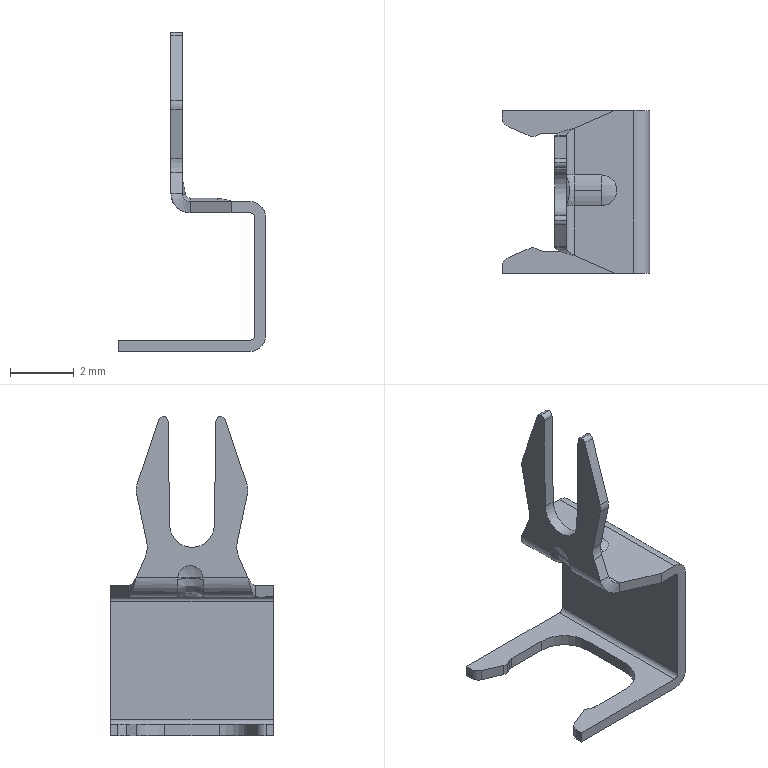Part | STEP file | LATCH | 1 solid | 68 faces | box 4.62 x 5.1 x 10 mm | volume 18.37 mm3 | cylinder 29 | plane 29 | spline 10 | commonest cylinder face diameters 0.3 x6 1 x4 1.4 x3 0.4 x2 0.494 x2 0.5 x2